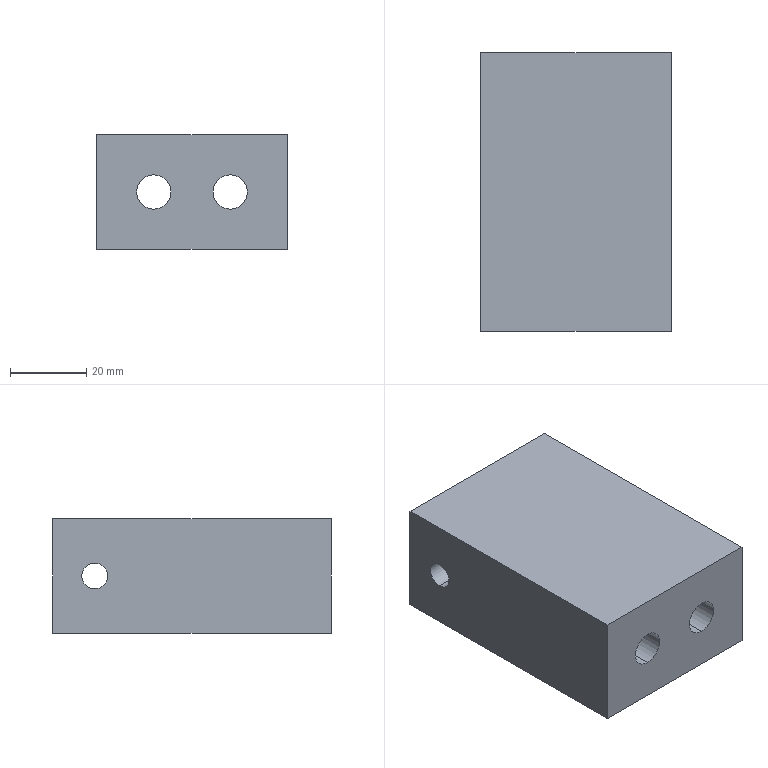Part | STEP file | HXGR200008-05-02 | 1 solid | 22 faces | box 50 x 73 x 30 mm | volume 90409 mm3 | cylinder 14 | plane 8 | commonest cylinder face diameters 6.8 x6 9 x4 15 x4
STEP:
#1=CARTESIAN_POINT('',(25.,25.5,-3.4));
#2=VERTEX_POINT('',#1);
#3=CARTESIAN_POINT('',(25.,25.5,3.4));
#4=VERTEX_POINT('',#3);
#5=CARTESIAN_POINT('',(25.,25.5,0.));
#6=DIRECTION('',(-1.,0.,0.));
#7=DIRECTION('',(0.,0.,1.));
#8=AXIS2_PLACEMENT_3D('',#5,#6,#7);
#9=CIRCLE('',#8,3.4);
#10=EDGE_CURVE('',#2,#4,#9,.T.);
#11=ORIENTED_EDGE('',*,*,#10,.F.);
#12=CARTESIAN_POINT('',(16.685,25.5,-3.4));
#13=VERTEX_POINT('',#12);
#14=CARTESIAN_POINT('',(-25.,25.5,-3.4));
#15=DIRECTION('',(-1.,0.,0.));
#16=VECTOR('',#15,1000.);
#17=LINE('',#14,#16);
#18=EDGE_CURVE('',#2,#13,#17,.T.);
#19=ORIENTED_EDGE('',*,*,#18,.T.);
#20=CARTESIAN_POINT('',(16.685,25.5,3.4));
#21=VERTEX_POINT('',#20);
#22=CARTESIAN_POINT('',(16.685,25.5,3.4));
#23=CARTESIAN_POINT('',(16.685,25.272,3.4));
#24=CARTESIAN_POINT('',(16.697,25.048,3.377));
#25=CARTESIAN_POINT('',(16.741,24.61,3.289));
#26=CARTESIAN_POINT('',(16.773,24.392,3.222));
#27=CARTESIAN_POINT('',(16.852,23.983,3.051));
#28=CARTESIAN_POINT('',(16.898,23.789,2.946));
#29=CARTESIAN_POINT('',(16.998,23.422,2.7));
#30=CARTESIAN_POINT('',(17.052,23.251,2.559));
#31=CARTESIAN_POINT('',(17.156,22.942,2.25));
#32=CARTESIAN_POINT('',(17.209,22.801,2.079));
#33=CARTESIAN_POINT('',(17.305,22.554,1.711));
#34=CARTESIAN_POINT('',(17.348,22.449,1.517));
#35=CARTESIAN_POINT('',(17.421,22.278,1.109));
#36=CARTESIAN_POINT('',(17.45,22.211,0.8911));
#37=CARTESIAN_POINT('',(17.49,22.122,0.4505));
#38=CARTESIAN_POINT('',(17.5,22.1,0.2275));
#39=CARTESIAN_POINT('',(17.5,22.1,-0.2236));
#40=CARTESIAN_POINT('',(17.49,22.123,-0.452));
#41=CARTESIAN_POINT('',(17.45,22.211,-0.8913));
#42=CARTESIAN_POINT('',(17.421,22.277,-1.106));
#43=CARTESIAN_POINT('',(17.347,22.45,-1.52));
#44=CARTESIAN_POINT('',(17.304,22.556,-1.715));
#45=CARTESIAN_POINT('',(17.208,22.802,-2.08));
#46=CARTESIAN_POINT('',(17.156,22.944,-2.253));
#47=CARTESIAN_POINT('',(17.051,23.254,-2.562));
#48=CARTESIAN_POINT('',(16.998,23.423,-2.701));
#49=CARTESIAN_POINT('',(16.898,23.79,-2.947));
#50=CARTESIAN_POINT('',(16.851,23.987,-3.053));
#51=CARTESIAN_POINT('',(16.773,24.394,-3.223));
#52=CARTESIAN_POINT('',(16.741,24.607,-3.289));
#53=CARTESIAN_POINT('',(16.696,25.052,-3.378));
#54=CARTESIAN_POINT('',(16.685,25.275,-3.4));
#55=CARTESIAN_POINT('',(16.685,25.5,-3.4));
#56=B_SPLINE_CURVE_WITH_KNOTS('',3,(#22,#23,#24,#25,#26,#27,#28,#29,#30,#31,#32,#33,#34,#35,#36,#37,#38,#39,#40,#41,#42,#43,#44,#45,#46,#47,#48,#49,#50,#51,#52,#53,#54,#55),.UNSPECIFIED.,.F.,.F.,(4,2,2,2,2,2,2,2,2,2,2,2,2,2,2,2,4),(0.,0.0006736,0.001347,0.002021,0.002695,0.003368,0.004042,0.004715,0.005389,0.006063,0.006736,0.00741,0.008084,0.008757,0.009431,0.0101,0.01078),.UNSPECIFIED.);
#57=EDGE_CURVE('',#21,#13,#56,.T.);
#58=ORIENTED_EDGE('',*,*,#57,.F.);
#59=CARTESIAN_POINT('',(-25.,25.5,3.4));
#60=DIRECTION('',(-1.,0.,0.));
#61=VECTOR('',#60,1000.);
#62=LINE('',#59,#61);
#63=EDGE_CURVE('',#4,#21,#62,.T.);
#64=ORIENTED_EDGE('',*,*,#63,.F.);
#65=EDGE_LOOP('',(#11,#19,#58,#64));
#66=FACE_OUTER_BOUND('',#65,.T.);
#67=CARTESIAN_POINT('',(-25.,25.5,0.));
#68=DIRECTION('',(-1.,0.,0.));
#69=DIRECTION('',(0.,0.,1.));
#70=AXIS2_PLACEMENT_3D('',#67,#68,#69);
#71=CYLINDRICAL_SURFACE('',#70,3.4);
#72=ADVANCED_FACE('',(#66),#71,.F.);
#73=CARTESIAN_POINT('',(-16.685,25.5,-3.4));
#74=VERTEX_POINT('',#73);
#75=CARTESIAN_POINT('',(-16.685,25.5,3.4));
#76=VERTEX_POINT('',#75);
#77=CARTESIAN_POINT('',(-16.685,25.5,-3.4));
#78=CARTESIAN_POINT('',(-16.685,25.276,-3.4));
#79=CARTESIAN_POINT('',(-16.697,25.048,-3.377));
#80=CARTESIAN_POINT('',(-16.741,24.607,-3.288));
#81=CARTESIAN_POINT('',(-16.773,24.394,-3.223));
#82=CARTESIAN_POINT('',(-16.852,23.983,-3.051));
#83=CARTESIAN_POINT('',(-16.899,23.787,-2.945));
#84=CARTESIAN_POINT('',(-16.998,23.422,-2.7));
#85=CARTESIAN_POINT('',(-17.052,23.251,-2.559));
#86=CARTESIAN_POINT('',(-17.157,22.94,-2.248));
#87=CARTESIAN_POINT('',(-17.208,22.801,-2.079));
#88=CARTESIAN_POINT('',(-17.304,22.556,-1.714));
#89=CARTESIAN_POINT('',(-17.348,22.449,-1.516));
#90=CARTESIAN_POINT('',(-17.421,22.278,-1.107));
#91=CARTESIAN_POINT('',(-17.45,22.212,-0.8946));
#92=CARTESIAN_POINT('',(-17.49,22.123,-0.4535));
#93=CARTESIAN_POINT('',(-17.5,22.1,-0.2259));
#94=CARTESIAN_POINT('',(-17.5,22.1,0.223));
#95=CARTESIAN_POINT('',(-17.49,22.122,0.4485));
#96=CARTESIAN_POINT('',(-17.45,22.211,0.8921));
#97=CARTESIAN_POINT('',(-17.421,22.277,1.105));
#98=CARTESIAN_POINT('',(-17.348,22.449,1.516));
#99=CARTESIAN_POINT('',(-17.304,22.556,1.714));
#100=CARTESIAN_POINT('',(-17.208,22.801,2.08));
#101=CARTESIAN_POINT('',(-17.157,22.94,2.249));
#102=CARTESIAN_POINT('',(-17.051,23.253,2.561));
#103=CARTESIAN_POINT('',(-16.998,23.423,2.701));
#104=CARTESIAN_POINT('',(-16.899,23.787,2.945));
#105=CARTESIAN_POINT('',(-16.852,23.983,3.051));
#106=CARTESIAN_POINT('',(-16.773,24.394,3.223));
#107=CARTESIAN_POINT('',(-16.741,24.606,3.288));
#108=CARTESIAN_POINT('',(-16.697,25.044,3.377));
#109=CARTESIAN_POINT('',(-16.685,25.272,3.4));
#110=CARTESIAN_POINT('',(-16.685,25.5,3.4));
#111=B_SPLINE_CURVE_WITH_KNOTS('',3,(#77,#78,#79,#80,#81,#82,#83,#84,#85,#86,#87,#88,#89,#90,#91,#92,#93,#94,#95,#96,#97,#98,#99,#100,#101,#102,#103,#104,#105,#106,#107,#108,#109,#110),.UNSPECIFIED.,.F.,.F.,(4,2,2,2,2,2,2,2,2,2,2,2,2,2,2,2,4),(0.01078,0.01145,0.01212,0.0128,0.01347,0.01414,0.01482,0.01549,0.01616,0.01683,0.01751,0.01818,0.01885,0.01953,0.0202,0.02087,0.02154),.UNSPECIFIED.);
#112=EDGE_CURVE('',#74,#76,#111,.T.);
#113=ORIENTED_EDGE('',*,*,#112,.F.);
#114=CARTESIAN_POINT('',(-25.,25.5,-3.4));
#115=VERTEX_POINT('',#114);
#116=CARTESIAN_POINT('',(-25.,25.5,-3.4));
#117=DIRECTION('',(-1.,0.,0.));
#118=VECTOR('',#117,1000.);
#119=LINE('',#116,#118);
#120=EDGE_CURVE('',#74,#115,#119,.T.);
#121=ORIENTED_EDGE('',*,*,#120,.T.);
#122=CARTESIAN_POINT('',(-25.,25.5,3.4));
#123=VERTEX_POINT('',#122);
#124=CARTESIAN_POINT('',(-25.,25.5,0.));
#125=DIRECTION('',(-1.,0.,0.));
#126=DIRECTION('',(0.,0.,1.));
#127=AXIS2_PLACEMENT_3D('',#124,#125,#126);
#128=CIRCLE('',#127,3.4);
#129=EDGE_CURVE('',#115,#123,#128,.T.);
#130=ORIENTED_EDGE('',*,*,#129,.T.);
#131=CARTESIAN_POINT('',(-25.,25.5,3.4));
#132=DIRECTION('',(-1.,0.,0.));
#133=VECTOR('',#132,1000.);
#134=LINE('',#131,#133);
#135=EDGE_CURVE('',#76,#123,#134,.T.);
#136=ORIENTED_EDGE('',*,*,#135,.F.);
#137=EDGE_LOOP('',(#113,#121,#130,#136));
#138=FACE_OUTER_BOUND('',#137,.T.);
#139=CARTESIAN_POINT('',(-25.,25.5,0.));
#140=DIRECTION('',(-1.,0.,0.));
#141=DIRECTION('',(0.,0.,1.));
#142=AXIS2_PLACEMENT_3D('',#139,#140,#141);
#143=CYLINDRICAL_SURFACE('',#142,3.4);
#144=ADVANCED_FACE('',(#138),#143,.F.);
#145=CARTESIAN_POINT('',(3.315,25.5,-3.4));
#146=VERTEX_POINT('',#145);
#147=CARTESIAN_POINT('',(3.315,25.5,3.4));
#148=VERTEX_POINT('',#147);
#149=CARTESIAN_POINT('',(3.315,25.5,-3.4));
#150=CARTESIAN_POINT('',(3.315,25.276,-3.4));
#151=CARTESIAN_POINT('',(3.303,25.048,-3.377));
#152=CARTESIAN_POINT('',(3.259,24.607,-3.288));
#153=CARTESIAN_POINT('',(3.227,24.394,-3.223));
#154=CARTESIAN_POINT('',(3.148,23.983,-3.051));
#155=CARTESIAN_POINT('',(3.101,23.787,-2.945));
#156=CARTESIAN_POINT('',(3.002,23.422,-2.7));
#157=CARTESIAN_POINT('',(2.948,23.251,-2.559));
#158=CARTESIAN_POINT('',(2.843,22.94,-2.248));
#159=CARTESIAN_POINT('',(2.792,22.801,-2.079));
#160=CARTESIAN_POINT('',(2.696,22.556,-1.714));
#161=CARTESIAN_POINT('',(2.652,22.449,-1.516));
#162=CARTESIAN_POINT('',(2.579,22.278,-1.107));
#163=CARTESIAN_POINT('',(2.55,22.212,-0.8946));
#164=CARTESIAN_POINT('',(2.51,22.123,-0.4535));
#165=CARTESIAN_POINT('',(2.5,22.1,-0.2259));
#166=CARTESIAN_POINT('',(2.5,22.1,0.223));
#167=CARTESIAN_POINT('',(2.51,22.122,0.4485));
#168=CARTESIAN_POINT('',(2.55,22.211,0.8921));
#169=CARTESIAN_POINT('',(2.579,22.277,1.105));
#170=CARTESIAN_POINT('',(2.652,22.449,1.516));
#171=CARTESIAN_POINT('',(2.696,22.556,1.714));
#172=CARTESIAN_POINT('',(2.792,22.801,2.08));
#173=CARTESIAN_POINT('',(2.843,22.94,2.249));
#174=CARTESIAN_POINT('',(2.949,23.253,2.561));
#175=CARTESIAN_POINT('',(3.002,23.423,2.701));
#176=CARTESIAN_POINT('',(3.101,23.787,2.945));
#177=CARTESIAN_POINT('',(3.148,23.983,3.051));
#178=CARTESIAN_POINT('',(3.227,24.394,3.223));
#179=CARTESIAN_POINT('',(3.259,24.606,3.288));
#180=CARTESIAN_POINT('',(3.303,25.044,3.377));
#181=CARTESIAN_POINT('',(3.315,25.272,3.4));
#182=CARTESIAN_POINT('',(3.315,25.5,3.4));
#183=B_SPLINE_CURVE_WITH_KNOTS('',3,(#149,#150,#151,#152,#153,#154,#155,#156,#157,#158,#159,#160,#161,#162,#163,#164,#165,#166,#167,#168,#169,#170,#171,#172,#173,#174,#175,#176,#177,#178,#179,#180,#181,#182),.UNSPECIFIED.,.F.,.F.,(4,2,2,2,2,2,2,2,2,2,2,2,2,2,2,2,4),(0.01078,0.01145,0.01212,0.0128,0.01347,0.01414,0.01482,0.01549,0.01616,0.01683,0.01751,0.01818,0.01885,0.01953,0.0202,0.02087,0.02154),.UNSPECIFIED.);
#184=EDGE_CURVE('',#146,#148,#183,.T.);
#185=ORIENTED_EDGE('',*,*,#184,.F.);
#186=CARTESIAN_POINT('',(-3.315,25.5,-3.4));
#187=VERTEX_POINT('',#186);
#188=CARTESIAN_POINT('',(-25.,25.5,-3.4));
#189=DIRECTION('',(-1.,0.,0.));
#190=VECTOR('',#189,1000.);
#191=LINE('',#188,#190);
#192=EDGE_CURVE('',#146,#187,#191,.T.);
#193=ORIENTED_EDGE('',*,*,#192,.T.);
#194=CARTESIAN_POINT('',(-3.315,25.5,3.4));
#195=VERTEX_POINT('',#194);
#196=CARTESIAN_POINT('',(-3.315,25.5,3.4));
#197=CARTESIAN_POINT('',(-3.315,25.272,3.4));
#198=CARTESIAN_POINT('',(-3.303,25.048,3.377));
#199=CARTESIAN_POINT('',(-3.259,24.61,3.289));
#200=CARTESIAN_POINT('',(-3.227,24.392,3.222));
#201=CARTESIAN_POINT('',(-3.148,23.983,3.051));
#202=CARTESIAN_POINT('',(-3.102,23.789,2.946));
#203=CARTESIAN_POINT('',(-3.002,23.422,2.7));
#204=CARTESIAN_POINT('',(-2.948,23.251,2.559));
#205=CARTESIAN_POINT('',(-2.844,22.942,2.25));
#206=CARTESIAN_POINT('',(-2.791,22.801,2.079));
#207=CARTESIAN_POINT('',(-2.695,22.554,1.711));
#208=CARTESIAN_POINT('',(-2.652,22.449,1.517));
#209=CARTESIAN_POINT('',(-2.579,22.278,1.109));
#210=CARTESIAN_POINT('',(-2.55,22.211,0.8911));
#211=CARTESIAN_POINT('',(-2.51,22.122,0.4505));
#212=CARTESIAN_POINT('',(-2.5,22.1,0.2275));
#213=CARTESIAN_POINT('',(-2.5,22.1,-0.2236));
#214=CARTESIAN_POINT('',(-2.51,22.123,-0.452));
#215=CARTESIAN_POINT('',(-2.55,22.211,-0.8913));
#216=CARTESIAN_POINT('',(-2.579,22.277,-1.106));
#217=CARTESIAN_POINT('',(-2.653,22.45,-1.52));
#218=CARTESIAN_POINT('',(-2.696,22.556,-1.715));
#219=CARTESIAN_POINT('',(-2.792,22.802,-2.08));
#220=CARTESIAN_POINT('',(-2.844,22.944,-2.253));
#221=CARTESIAN_POINT('',(-2.949,23.254,-2.562));
#222=CARTESIAN_POINT('',(-3.002,23.423,-2.701));
#223=CARTESIAN_POINT('',(-3.102,23.79,-2.947));
#224=CARTESIAN_POINT('',(-3.149,23.987,-3.053));
#225=CARTESIAN_POINT('',(-3.227,24.394,-3.223));
#226=CARTESIAN_POINT('',(-3.259,24.607,-3.289));
#227=CARTESIAN_POINT('',(-3.304,25.052,-3.378));
#228=CARTESIAN_POINT('',(-3.315,25.275,-3.4));
#229=CARTESIAN_POINT('',(-3.315,25.5,-3.4));
#230=B_SPLINE_CURVE_WITH_KNOTS('',3,(#196,#197,#198,#199,#200,#201,#202,#203,#204,#205,#206,#207,#208,#209,#210,#211,#212,#213,#214,#215,#216,#217,#218,#219,#220,#221,#222,#223,#224,#225,#226,#227,#228,#229),.UNSPECIFIED.,.F.,.F.,(4,2,2,2,2,2,2,2,2,2,2,2,2,2,2,2,4),(0.,0.0006736,0.001347,0.002021,0.002695,0.003368,0.004042,0.004715,0.005389,0.006063,0.006736,0.00741,0.008084,0.008757,0.009431,0.0101,0.01078),.UNSPECIFIED.);
#231=EDGE_CURVE('',#195,#187,#230,.T.);
#232=ORIENTED_EDGE('',*,*,#231,.F.);
#233=CARTESIAN_POINT('',(-25.,25.5,3.4));
#234=DIRECTION('',(-1.,0.,0.));
#235=VECTOR('',#234,1000.);
#236=LINE('',#233,#235);
#237=EDGE_CURVE('',#148,#195,#236,.T.);
#238=ORIENTED_EDGE('',*,*,#237,.F.);
#239=EDGE_LOOP('',(#185,#193,#232,#238));
#240=FACE_OUTER_BOUND('',#239,.T.);
#241=CARTESIAN_POINT('',(-25.,25.5,0.));
#242=DIRECTION('',(-1.,0.,0.));
#243=DIRECTION('',(0.,0.,1.));
#244=AXIS2_PLACEMENT_3D('',#241,#242,#243);
#245=CYLINDRICAL_SURFACE('',#244,3.4);
#246=ADVANCED_FACE('',(#240),#245,.F.);
#247=CARTESIAN_POINT('',(-16.685,25.5,3.4));
#248=CARTESIAN_POINT('',(-16.685,25.728,3.4));
#249=CARTESIAN_POINT('',(-16.697,25.952,3.377));
#250=CARTESIAN_POINT('',(-16.741,26.39,3.289));
#251=CARTESIAN_POINT('',(-16.773,26.608,3.222));
#252=CARTESIAN_POINT('',(-16.852,27.017,3.051));
#253=CARTESIAN_POINT('',(-16.898,27.211,2.946));
#254=CARTESIAN_POINT('',(-16.998,27.578,2.7));
#255=CARTESIAN_POINT('',(-17.052,27.749,2.559));
#256=CARTESIAN_POINT('',(-17.156,28.058,2.25));
#257=CARTESIAN_POINT('',(-17.209,28.199,2.079));
#258=CARTESIAN_POINT('',(-17.305,28.446,1.711));
#259=CARTESIAN_POINT('',(-17.348,28.551,1.517));
#260=CARTESIAN_POINT('',(-17.421,28.722,1.109));
#261=CARTESIAN_POINT('',(-17.45,28.789,0.8911));
#262=CARTESIAN_POINT('',(-17.49,28.878,0.4505));
#263=CARTESIAN_POINT('',(-17.5,28.9,0.2275));
#264=CARTESIAN_POINT('',(-17.5,28.9,-0.2236));
#265=CARTESIAN_POINT('',(-17.49,28.877,-0.452));
#266=CARTESIAN_POINT('',(-17.45,28.789,-0.8913));
#267=CARTESIAN_POINT('',(-17.421,28.723,-1.106));
#268=CARTESIAN_POINT('',(-17.347,28.55,-1.52));
#269=CARTESIAN_POINT('',(-17.304,28.444,-1.715));
#270=CARTESIAN_POINT('',(-17.208,28.198,-2.08));
#271=CARTESIAN_POINT('',(-17.156,28.056,-2.253));
#272=CARTESIAN_POINT('',(-17.051,27.746,-2.562));
#273=CARTESIAN_POINT('',(-16.998,27.577,-2.701));
#274=CARTESIAN_POINT('',(-16.898,27.21,-2.947));
#275=CARTESIAN_POINT('',(-16.851,27.013,-3.053));
#276=CARTESIAN_POINT('',(-16.773,26.606,-3.223));
#277=CARTESIAN_POINT('',(-16.741,26.393,-3.289));
#278=CARTESIAN_POINT('',(-16.696,25.948,-3.378));
#279=CARTESIAN_POINT('',(-16.685,25.725,-3.4));
#280=CARTESIAN_POINT('',(-16.685,25.5,-3.4));
#281=B_SPLINE_CURVE_WITH_KNOTS('',3,(#247,#248,#249,#250,#251,#252,#253,#254,#255,#256,#257,#258,#259,#260,#261,#262,#263,#264,#265,#266,#267,#268,#269,#270,#271,#272,#273,#274,#275,#276,#277,#278,#279,#280),.UNSPECIFIED.,.F.,.F.,(4,2,2,2,2,2,2,2,2,2,2,2,2,2,2,2,4),(0.,0.0006736,0.001347,0.002021,0.002695,0.003368,0.004042,0.004715,0.005389,0.006063,0.006736,0.00741,0.008084,0.008757,0.009431,0.0101,0.01078),.UNSPECIFIED.);
#282=EDGE_CURVE('',#76,#74,#281,.T.);
#283=ORIENTED_EDGE('',*,*,#282,.T.);
#284=ORIENTED_EDGE('',*,*,#112,.T.);
#285=EDGE_LOOP('',(#283,#284));
#286=FACE_BOUND('',#285,.T.);
#287=CARTESIAN_POINT('',(-10.,-3.5,-7.5));
#288=VERTEX_POINT('',#287);
#289=CARTESIAN_POINT('',(-10.,-3.5,7.5));
#290=VERTEX_POINT('',#289);
#291=CARTESIAN_POINT('',(-10.,-3.5,0.));
#292=DIRECTION('',(0.,1.,0.));
#293=DIRECTION('',(0.,0.,1.));
#294=AXIS2_PLACEMENT_3D('',#291,#292,#293);
#295=CIRCLE('',#294,7.5);
#296=EDGE_CURVE('',#288,#290,#295,.T.);
#297=ORIENTED_EDGE('',*,*,#296,.F.);
#298=CARTESIAN_POINT('',(-10.,36.5,-7.5));
#299=VERTEX_POINT('',#298);
#300=CARTESIAN_POINT('',(-10.,36.5,-7.5));
#301=DIRECTION('',(0.,1.,0.));
#302=VECTOR('',#301,1000.);
#303=LINE('',#300,#302);
#304=EDGE_CURVE('',#288,#299,#303,.T.);
#305=ORIENTED_EDGE('',*,*,#304,.T.);
#306=CARTESIAN_POINT('',(-10.,36.5,7.5));
#307=VERTEX_POINT('',#306);
#308=CARTESIAN_POINT('',(-10.,36.5,0.));
#309=DIRECTION('',(0.,1.,0.));
#310=DIRECTION('',(0.,0.,1.));
#311=AXIS2_PLACEMENT_3D('',#308,#309,#310);
#312=CIRCLE('',#311,7.5);
#313=EDGE_CURVE('',#299,#307,#312,.T.);
#314=ORIENTED_EDGE('',*,*,#313,.T.);
#315=CARTESIAN_POINT('',(-10.,36.5,7.5));
#316=DIRECTION('',(0.,1.,0.));
#317=VECTOR('',#316,1000.);
#318=LINE('',#315,#317);
#319=EDGE_CURVE('',#290,#307,#318,.T.);
#320=ORIENTED_EDGE('',*,*,#319,.F.);
#321=EDGE_LOOP('',(#297,#305,#314,#320));
#322=FACE_OUTER_BOUND('',#321,.T.);
#323=CARTESIAN_POINT('',(-10.,36.5,0.));
#324=DIRECTION('',(0.,1.,0.));
#325=DIRECTION('',(0.,0.,1.));
#326=AXIS2_PLACEMENT_3D('',#323,#324,#325);
#327=CYLINDRICAL_SURFACE('',#326,7.5);
#328=ADVANCED_FACE('',(#286,#322),#327,.F.);
#329=CARTESIAN_POINT('',(-10.,-36.5,-4.5));
#330=VERTEX_POINT('',#329);
#331=CARTESIAN_POINT('',(-10.,-36.5,4.5));
#332=VERTEX_POINT('',#331);
#333=CARTESIAN_POINT('',(-10.,-36.5,0.));
#334=DIRECTION('',(0.,1.,0.));
#335=DIRECTION('',(0.,0.,1.));
#336=AXIS2_PLACEMENT_3D('',#333,#334,#335);
#337=CIRCLE('',#336,4.5);
#338=EDGE_CURVE('',#330,#332,#337,.T.);
#339=ORIENTED_EDGE('',*,*,#338,.F.);
#340=CARTESIAN_POINT('',(-10.,-3.5,-4.5));
#341=VERTEX_POINT('',#340);
#342=CARTESIAN_POINT('',(-10.,36.5,-4.5));
#343=DIRECTION('',(0.,1.,0.));
#344=VECTOR('',#343,1000.);
#345=LINE('',#342,#344);
#346=EDGE_CURVE('',#330,#341,#345,.T.);
#347=ORIENTED_EDGE('',*,*,#346,.T.);
#348=CARTESIAN_POINT('',(-10.,-3.5,4.5));
#349=VERTEX_POINT('',#348);
#350=CARTESIAN_POINT('',(-10.,-3.5,0.));
#351=DIRECTION('',(0.,1.,0.));
#352=DIRECTION('',(0.,0.,1.));
#353=AXIS2_PLACEMENT_3D('',#350,#351,#352);
#354=CIRCLE('',#353,4.5);
#355=EDGE_CURVE('',#341,#349,#354,.T.);
#356=ORIENTED_EDGE('',*,*,#355,.T.);
#357=CARTESIAN_POINT('',(-10.,36.5,4.5));
#358=DIRECTION('',(0.,1.,0.));
#359=VECTOR('',#358,1000.);
#360=LINE('',#357,#359);
#361=EDGE_CURVE('',#332,#349,#360,.T.);
#362=ORIENTED_EDGE('',*,*,#361,.F.);
#363=EDGE_LOOP('',(#339,#347,#356,#362));
#364=FACE_OUTER_BOUND('',#363,.T.);
#365=CARTESIAN_POINT('',(-10.,36.5,0.));
#366=DIRECTION('',(0.,1.,0.));
#367=DIRECTION('',(0.,0.,1.));
#368=AXIS2_PLACEMENT_3D('',#365,#366,#367);
#369=CYLINDRICAL_SURFACE('',#368,4.5);
#370=ADVANCED_FACE('',(#364),#369,.F.);
#371=CARTESIAN_POINT('',(3.315,25.5,3.4));
#372=CARTESIAN_POINT('',(3.315,25.728,3.4));
#373=CARTESIAN_POINT('',(3.303,25.952,3.377));
#374=CARTESIAN_POINT('',(3.259,26.39,3.289));
#375=CARTESIAN_POINT('',(3.227,26.608,3.222));
#376=CARTESIAN_POINT('',(3.148,27.017,3.051));
#377=CARTESIAN_POINT('',(3.102,27.211,2.946));
#378=CARTESIAN_POINT('',(3.002,27.578,2.7));
#379=CARTESIAN_POINT('',(2.948,27.749,2.559));
#380=CARTESIAN_POINT('',(2.844,28.058,2.25));
#381=CARTESIAN_POINT('',(2.791,28.199,2.079));
#382=CARTESIAN_POINT('',(2.695,28.446,1.711));
#383=CARTESIAN_POINT('',(2.652,28.551,1.517));
#384=CARTESIAN_POINT('',(2.579,28.722,1.109));
#385=CARTESIAN_POINT('',(2.55,28.789,0.8911));
#386=CARTESIAN_POINT('',(2.51,28.878,0.4505));
#387=CARTESIAN_POINT('',(2.5,28.9,0.2275));
#388=CARTESIAN_POINT('',(2.5,28.9,-0.2236));
#389=CARTESIAN_POINT('',(2.51,28.877,-0.452));
#390=CARTESIAN_POINT('',(2.55,28.789,-0.8913));
#391=CARTESIAN_POINT('',(2.579,28.723,-1.106));
#392=CARTESIAN_POINT('',(2.653,28.55,-1.52));
#393=CARTESIAN_POINT('',(2.696,28.444,-1.715));
#394=CARTESIAN_POINT('',(2.792,28.198,-2.08));
#395=CARTESIAN_POINT('',(2.844,28.056,-2.253));
#396=CARTESIAN_POINT('',(2.949,27.746,-2.562));
#397=CARTESIAN_POINT('',(3.002,27.577,-2.701));
#398=CARTESIAN_POINT('',(3.102,27.21,-2.947));
#399=CARTESIAN_POINT('',(3.149,27.013,-3.053));
#400=CARTESIAN_POINT('',(3.227,26.606,-3.223));
#401=CARTESIAN_POINT('',(3.259,26.393,-3.289));
#402=CARTESIAN_POINT('',(3.304,25.948,-3.378));
#403=CARTESIAN_POINT('',(3.315,25.725,-3.4));
#404=CARTESIAN_POINT('',(3.315,25.5,-3.4));
#405=B_SPLINE_CURVE_WITH_KNOTS('',3,(#371,#372,#373,#374,#375,#376,#377,#378,#379,#380,#381,#382,#383,#384,#385,#386,#387,#388,#389,#390,#391,#392,#393,#394,#395,#396,#397,#398,#399,#400,#401,#402,#403,#404),.UNSPECIFIED.,.F.,.F.,(4,2,2,2,2,2,2,2,2,2,2,2,2,2,2,2,4),(0.,0.0006736,0.001347,0.002021,0.002695,0.003368,0.004042,0.004715,0.005389,0.006063,0.006736,0.00741,0.008084,0.008757,0.009431,0.0101,0.01078),.UNSPECIFIED.);
#406=EDGE_CURVE('',#148,#146,#405,.T.);
#407=ORIENTED_EDGE('',*,*,#406,.T.);
#408=ORIENTED_EDGE('',*,*,#184,.T.);
#409=EDGE_LOOP('',(#407,#408));
#410=FACE_BOUND('',#409,.T.);
#411=CARTESIAN_POINT('',(10.,-3.5,-7.5));
#412=VERTEX_POINT('',#411);
#413=CARTESIAN_POINT('',(10.,-3.5,7.5));
#414=VERTEX_POINT('',#413);
#415=CARTESIAN_POINT('',(10.,-3.5,0.));
#416=DIRECTION('',(0.,1.,0.));
#417=DIRECTION('',(0.,0.,1.));
#418=AXIS2_PLACEMENT_3D('',#415,#416,#417);
#419=CIRCLE('',#418,7.5);
#420=EDGE_CURVE('',#412,#414,#419,.T.);
#421=ORIENTED_EDGE('',*,*,#420,.F.);
#422=CARTESIAN_POINT('',(10.,36.5,-7.5));
#423=VERTEX_POINT('',#422);
#424=CARTESIAN_POINT('',(10.,36.5,-7.5));
#425=DIRECTION('',(0.,1.,0.));
#426=VECTOR('',#425,1000.);
#427=LINE('',#424,#426);
#428=EDGE_CURVE('',#412,#423,#427,.T.);
#429=ORIENTED_EDGE('',*,*,#428,.T.);
#430=CARTESIAN_POINT('',(10.,36.5,7.5));
#431=VERTEX_POINT('',#430);
#432=CARTESIAN_POINT('',(10.,36.5,0.));
#433=DIRECTION('',(0.,1.,0.));
#434=DIRECTION('',(0.,0.,1.));
#435=AXIS2_PLACEMENT_3D('',#432,#433,#434);
#436=CIRCLE('',#435,7.5);
#437=EDGE_CURVE('',#423,#431,#436,.T.);
#438=ORIENTED_EDGE('',*,*,#437,.T.);
#439=CARTESIAN_POINT('',(10.,36.5,7.5));
#440=DIRECTION('',(0.,1.,0.));
#441=VECTOR('',#440,1000.);
#442=LINE('',#439,#441);
#443=EDGE_CURVE('',#414,#431,#442,.T.);
#444=ORIENTED_EDGE('',*,*,#443,.F.);
#445=EDGE_LOOP('',(#421,#429,#438,#444));
#446=FACE_OUTER_BOUND('',#445,.T.);
#447=CARTESIAN_POINT('',(10.,36.5,0.));
#448=DIRECTION('',(0.,1.,0.));
#449=DIRECTION('',(0.,0.,1.));
#450=AXIS2_PLACEMENT_3D('',#447,#448,#449);
#451=CYLINDRICAL_SURFACE('',#450,7.5);
#452=ADVANCED_FACE('',(#410,#446),#451,.F.);
#453=CARTESIAN_POINT('',(10.,-36.5,-4.5));
#454=VERTEX_POINT('',#453);
#455=CARTESIAN_POINT('',(10.,-36.5,4.5));
#456=VERTEX_POINT('',#455);
#457=CARTESIAN_POINT('',(10.,-36.5,0.));
#458=DIRECTION('',(0.,1.,0.));
#459=DIRECTION('',(0.,0.,1.));
#460=AXIS2_PLACEMENT_3D('',#457,#458,#459);
#461=CIRCLE('',#460,4.5);
#462=EDGE_CURVE('',#454,#456,#461,.T.);
#463=ORIENTED_EDGE('',*,*,#462,.F.);
#464=CARTESIAN_POINT('',(10.,-3.5,-4.5));
#465=VERTEX_POINT('',#464);
#466=CARTESIAN_POINT('',(10.,36.5,-4.5));
#467=DIRECTION('',(0.,1.,0.));
#468=VECTOR('',#467,1000.);
#469=LINE('',#466,#468);
#470=EDGE_CURVE('',#454,#465,#469,.T.);
#471=ORIENTED_EDGE('',*,*,#470,.T.);
#472=CARTESIAN_POINT('',(10.,-3.5,4.5));
#473=VERTEX_POINT('',#472);
#474=CARTESIAN_POINT('',(10.,-3.5,0.));
#475=DIRECTION('',(0.,1.,0.));
#476=DIRECTION('',(0.,0.,1.));
#477=AXIS2_PLACEMENT_3D('',#474,#475,#476);
#478=CIRCLE('',#477,4.5);
#479=EDGE_CURVE('',#465,#473,#478,.T.);
#480=ORIENTED_EDGE('',*,*,#479,.T.);
#481=CARTESIAN_POINT('',(10.,36.5,4.5));
#482=DIRECTION('',(0.,1.,0.));
#483=VECTOR('',#482,1000.);
#484=LINE('',#481,#483);
#485=EDGE_CURVE('',#456,#473,#484,.T.);
#486=ORIENTED_EDGE('',*,*,#485,.F.);
#487=EDGE_LOOP('',(#463,#471,#480,#486));
#488=FACE_OUTER_BOUND('',#487,.T.);
#489=CARTESIAN_POINT('',(10.,36.5,0.));
#490=DIRECTION('',(0.,1.,0.));
#491=DIRECTION('',(0.,0.,1.));
#492=AXIS2_PLACEMENT_3D('',#489,#490,#491);
#493=CYLINDRICAL_SURFACE('',#492,4.5);
#494=ADVANCED_FACE('',(#488),#493,.F.);
#495=CARTESIAN_POINT('',(-25.,25.5,0.));
#496=DIRECTION('',(-1.,0.,0.));
#497=DIRECTION('',(0.,0.,1.));
#498=AXIS2_PLACEMENT_3D('',#495,#496,#497);
#499=CIRCLE('',#498,3.4);
#500=EDGE_CURVE('',#123,#115,#499,.T.);
#501=ORIENTED_EDGE('',*,*,#500,.F.);
#502=ORIENTED_EDGE('',*,*,#129,.F.);
#503=EDGE_LOOP('',(#501,#502));
#504=FACE_BOUND('',#503,.T.);
#505=CARTESIAN_POINT('',(-25.,36.5,-15.));
#506=VERTEX_POINT('',#505);
#507=CARTESIAN_POINT('',(-25.,-36.5,-15.));
#508=VERTEX_POINT('',#507);
#509=CARTESIAN_POINT('',(-25.,-36.5,-15.));
#510=DIRECTION('',(0.,-1.,0.));
#511=VECTOR('',#510,1000.);
#512=LINE('',#509,#511);
#513=EDGE_CURVE('',#506,#508,#512,.T.);
#514=ORIENTED_EDGE('',*,*,#513,.T.);
#515=CARTESIAN_POINT('',(-25.,-36.5,15.));
#516=VERTEX_POINT('',#515);
#517=CARTESIAN_POINT('',(-25.,-36.5,15.));
#518=DIRECTION('',(0.,0.,-1.));
#519=VECTOR('',#518,1000.);
#520=LINE('',#517,#519);
#521=EDGE_CURVE('',#516,#508,#520,.T.);
#522=ORIENTED_EDGE('',*,*,#521,.F.);
#523=CARTESIAN_POINT('',(-25.,36.5,15.));
#524=VERTEX_POINT('',#523);
#525=CARTESIAN_POINT('',(-25.,-36.5,15.));
#526=DIRECTION('',(0.,-1.,0.));
#527=VECTOR('',#526,1000.);
#528=LINE('',#525,#527);
#529=EDGE_CURVE('',#524,#516,#528,.T.);
#530=ORIENTED_EDGE('',*,*,#529,.F.);
#531=CARTESIAN_POINT('',(-25.,36.5,15.));
#532=DIRECTION('',(0.,0.,-1.));
#533=VECTOR('',#532,1000.);
#534=LINE('',#531,#533);
#535=EDGE_CURVE('',#524,#506,#534,.T.);
#536=ORIENTED_EDGE('',*,*,#535,.T.);
#537=EDGE_LOOP('',(#514,#522,#530,#536));
#538=FACE_OUTER_BOUND('',#537,.T.);
#539=CARTESIAN_POINT('',(-25.,-36.5,15.));
#540=DIRECTION('',(1.,0.,0.));
#541=DIRECTION('',(0.,0.,-1.));
#542=AXIS2_PLACEMENT_3D('',#539,#540,#541);
#543=PLANE('',#542);
#544=ADVANCED_FACE('',(#504,#538),#543,.F.);
#545=CARTESIAN_POINT('',(-10.,-36.5,0.));
#546=DIRECTION('',(0.,1.,0.));
#547=DIRECTION('',(0.,0.,1.));
#548=AXIS2_PLACEMENT_3D('',#545,#546,#547);
#549=CIRCLE('',#548,4.5);
#550=EDGE_CURVE('',#332,#330,#549,.T.);
#551=ORIENTED_EDGE('',*,*,#550,.T.);
#552=ORIENTED_EDGE('',*,*,#338,.T.);
#553=EDGE_LOOP('',(#551,#552));
#554=FACE_BOUND('',#553,.T.);
#555=CARTESIAN_POINT('',(10.,-36.5,0.));
#556=DIRECTION('',(0.,1.,0.));
#557=DIRECTION('',(0.,0.,1.));
#558=AXIS2_PLACEMENT_3D('',#555,#556,#557);
#559=CIRCLE('',#558,4.5);
#560=EDGE_CURVE('',#456,#454,#559,.T.);
#561=ORIENTED_EDGE('',*,*,#560,.T.);
#562=ORIENTED_EDGE('',*,*,#462,.T.);
#563=EDGE_LOOP('',(#561,#562));
#564=FACE_BOUND('',#563,.T.);
#565=CARTESIAN_POINT('',(25.,-36.5,-15.));
#566=VERTEX_POINT('',#565);
#567=CARTESIAN_POINT('',(25.,-36.5,-15.));
#568=DIRECTION('',(1.,0.,0.));
#569=VECTOR('',#568,1000.);
#570=LINE('',#567,#569);
#571=EDGE_CURVE('',#508,#566,#570,.T.);
#572=ORIENTED_EDGE('',*,*,#571,.T.);
#573=CARTESIAN_POINT('',(25.,-36.5,15.));
#574=VERTEX_POINT('',#573);
#575=CARTESIAN_POINT('',(25.,-36.5,15.));
#576=DIRECTION('',(0.,0.,-1.));
#577=VECTOR('',#576,1000.);
#578=LINE('',#575,#577);
#579=EDGE_CURVE('',#574,#566,#578,.T.);
#580=ORIENTED_EDGE('',*,*,#579,.F.);
#581=CARTESIAN_POINT('',(25.,-36.5,15.));
#582=DIRECTION('',(1.,0.,0.));
#583=VECTOR('',#582,1000.);
#584=LINE('',#581,#583);
#585=EDGE_CURVE('',#516,#574,#584,.T.);
#586=ORIENTED_EDGE('',*,*,#585,.F.);
#587=ORIENTED_EDGE('',*,*,#521,.T.);
#588=EDGE_LOOP('',(#572,#580,#586,#587));
#589=FACE_OUTER_BOUND('',#588,.T.);
#590=CARTESIAN_POINT('',(25.,-36.5,15.));
#591=DIRECTION('',(0.,1.,0.));
#592=DIRECTION('',(0.,0.,1.));
#593=AXIS2_PLACEMENT_3D('',#590,#591,#592);
#594=PLANE('',#593);
#595=ADVANCED_FACE('',(#554,#564,#589),#594,.F.);
#596=CARTESIAN_POINT('',(25.,25.5,0.));
#597=DIRECTION('',(-1.,0.,0.));
#598=DIRECTION('',(0.,0.,1.));
#599=AXIS2_PLACEMENT_3D('',#596,#597,#598);
#600=CIRCLE('',#599,3.4);
#601=EDGE_CURVE('',#4,#2,#600,.T.);
#602=ORIENTED_EDGE('',*,*,#601,.T.);
#603=ORIENTED_EDGE('',*,*,#10,.T.);
#604=EDGE_LOOP('',(#602,#603));
#605=FACE_BOUND('',#604,.T.);
#606=CARTESIAN_POINT('',(25.,36.5,-15.));
#607=VERTEX_POINT('',#606);
#608=CARTESIAN_POINT('',(25.,-36.5,-15.));
#609=DIRECTION('',(0.,1.,0.));
#610=VECTOR('',#609,1000.);
#611=LINE('',#608,#610);
#612=EDGE_CURVE('',#566,#607,#611,.T.);
#613=ORIENTED_EDGE('',*,*,#612,.T.);
#614=CARTESIAN_POINT('',(25.,36.5,15.));
#615=VERTEX_POINT('',#614);
#616=CARTESIAN_POINT('',(25.,36.5,15.));
#617=DIRECTION('',(0.,0.,-1.));
#618=VECTOR('',#617,1000.);
#619=LINE('',#616,#618);
#620=EDGE_CURVE('',#615,#607,#619,.T.);
#621=ORIENTED_EDGE('',*,*,#620,.F.);
#622=CARTESIAN_POINT('',(25.,-36.5,15.));
#623=DIRECTION('',(0.,1.,0.));
#624=VECTOR('',#623,1000.);
#625=LINE('',#622,#624);
#626=EDGE_CURVE('',#574,#615,#625,.T.);
#627=ORIENTED_EDGE('',*,*,#626,.F.);
#628=ORIENTED_EDGE('',*,*,#579,.T.);
#629=EDGE_LOOP('',(#613,#621,#627,#628));
#630=FACE_OUTER_BOUND('',#629,.T.);
#631=CARTESIAN_POINT('',(25.,-36.5,15.));
#632=DIRECTION('',(-1.,0.,0.));
#633=DIRECTION('',(0.,0.,1.));
#634=AXIS2_PLACEMENT_3D('',#631,#632,#633);
#635=PLANE('',#634);
#636=ADVANCED_FACE('',(#605,#630),#635,.F.);
#637=CARTESIAN_POINT('',(-10.,36.5,0.));
#638=DIRECTION('',(0.,1.,0.));
#639=DIRECTION('',(0.,0.,1.));
#640=AXIS2_PLACEMENT_3D('',#637,#638,#639);
#641=CIRCLE('',#640,7.5);
#642=EDGE_CURVE('',#307,#299,#641,.T.);
#643=ORIENTED_EDGE('',*,*,#642,.F.);
#644=ORIENTED_EDGE('',*,*,#313,.F.);
#645=EDGE_LOOP('',(#643,#644));
#646=FACE_BOUND('',#645,.T.);
#647=CARTESIAN_POINT('',(10.,36.5,0.));
#648=DIRECTION('',(0.,1.,0.));
#649=DIRECTION('',(0.,0.,1.));
#650=AXIS2_PLACEMENT_3D('',#647,#648,#649);
#651=CIRCLE('',#650,7.5);
#652=EDGE_CURVE('',#431,#423,#651,.T.);
#653=ORIENTED_EDGE('',*,*,#652,.F.);
#654=ORIENTED_EDGE('',*,*,#437,.F.);
#655=EDGE_LOOP('',(#653,#654));
#656=FACE_BOUND('',#655,.T.);
#657=CARTESIAN_POINT('',(25.,36.5,-15.));
#658=DIRECTION('',(-1.,0.,0.));
#659=VECTOR('',#658,1000.);
#660=LINE('',#657,#659);
#661=EDGE_CURVE('',#607,#506,#660,.T.);
#662=ORIENTED_EDGE('',*,*,#661,.T.);
#663=ORIENTED_EDGE('',*,*,#535,.F.);
#664=CARTESIAN_POINT('',(25.,36.5,15.));
#665=DIRECTION('',(-1.,0.,0.));
#666=VECTOR('',#665,1000.);
#667=LINE('',#664,#666);
#668=EDGE_CURVE('',#615,#524,#667,.T.);
#669=ORIENTED_EDGE('',*,*,#668,.F.);
#670=ORIENTED_EDGE('',*,*,#620,.T.);
#671=EDGE_LOOP('',(#662,#663,#669,#670));
#672=FACE_OUTER_BOUND('',#671,.T.);
#673=CARTESIAN_POINT('',(25.,36.5,15.));
#674=DIRECTION('',(0.,-1.,0.));
#675=DIRECTION('',(1.,0.,0.));
#676=AXIS2_PLACEMENT_3D('',#673,#674,#675);
#677=PLANE('',#676);
#678=ADVANCED_FACE('',(#646,#656,#672),#677,.F.);
#679=ORIENTED_EDGE('',*,*,#529,.T.);
#680=ORIENTED_EDGE('',*,*,#585,.T.);
#681=ORIENTED_EDGE('',*,*,#626,.T.);
#682=ORIENTED_EDGE('',*,*,#668,.T.);
#683=EDGE_LOOP('',(#679,#680,#681,#682));
#684=FACE_OUTER_BOUND('',#683,.T.);
#685=CARTESIAN_POINT('',(0.,0.,15.));
#686=DIRECTION('',(0.,0.,1.));
#687=DIRECTION('',(1.,0.,0.));
#688=AXIS2_PLACEMENT_3D('',#685,#686,#687);
#689=PLANE('',#688);
#690=ADVANCED_FACE('',(#684),#689,.T.);
#691=ORIENTED_EDGE('',*,*,#513,.F.);
#692=ORIENTED_EDGE('',*,*,#661,.F.);
#693=ORIENTED_EDGE('',*,*,#612,.F.);
#694=ORIENTED_EDGE('',*,*,#571,.F.);
#695=EDGE_LOOP('',(#691,#692,#693,#694));
#696=FACE_OUTER_BOUND('',#695,.T.);
#697=CARTESIAN_POINT('',(0.,0.,-15.));
#698=DIRECTION('',(0.,0.,1.));
#699=DIRECTION('',(1.,0.,0.));
#700=AXIS2_PLACEMENT_3D('',#697,#698,#699);
#701=PLANE('',#700);
#702=ADVANCED_FACE('',(#696),#701,.F.);
#703=ORIENTED_EDGE('',*,*,#470,.F.);
#704=ORIENTED_EDGE('',*,*,#560,.F.);
#705=ORIENTED_EDGE('',*,*,#485,.T.);
#706=CARTESIAN_POINT('',(10.,-3.5,0.));
#707=DIRECTION('',(0.,1.,0.));
#708=DIRECTION('',(0.,0.,1.));
#709=AXIS2_PLACEMENT_3D('',#706,#707,#708);
#710=CIRCLE('',#709,4.5);
#711=EDGE_CURVE('',#473,#465,#710,.T.);
#712=ORIENTED_EDGE('',*,*,#711,.T.);
#713=EDGE_LOOP('',(#703,#704,#705,#712));
#714=FACE_OUTER_BOUND('',#713,.T.);
#715=CARTESIAN_POINT('',(10.,36.5,0.));
#716=DIRECTION('',(0.,1.,0.));
#717=DIRECTION('',(0.,0.,1.));
#718=AXIS2_PLACEMENT_3D('',#715,#716,#717);
#719=CYLINDRICAL_SURFACE('',#718,4.5);
#720=ADVANCED_FACE('',(#714),#719,.F.);
#721=ORIENTED_EDGE('',*,*,#711,.F.);
#722=ORIENTED_EDGE('',*,*,#479,.F.);
#723=EDGE_LOOP('',(#721,#722));
#724=FACE_BOUND('',#723,.T.);
#725=CARTESIAN_POINT('',(10.,-3.5,0.));
#726=DIRECTION('',(0.,1.,0.));
#727=DIRECTION('',(0.,0.,1.));
#728=AXIS2_PLACEMENT_3D('',#725,#726,#727);
#729=CIRCLE('',#728,7.5);
#730=EDGE_CURVE('',#414,#412,#729,.T.);
#731=ORIENTED_EDGE('',*,*,#730,.T.);
#732=ORIENTED_EDGE('',*,*,#420,.T.);
#733=EDGE_LOOP('',(#731,#732));
#734=FACE_OUTER_BOUND('',#733,.T.);
#735=CARTESIAN_POINT('',(14.5,-3.5,0.));
#736=DIRECTION('',(0.,-1.,0.));
#737=DIRECTION('',(0.,0.,-1.));
#738=AXIS2_PLACEMENT_3D('',#735,#736,#737);
#739=PLANE('',#738);
#740=ADVANCED_FACE('',(#724,#734),#739,.F.);
#741=ORIENTED_EDGE('',*,*,#428,.F.);
#742=ORIENTED_EDGE('',*,*,#730,.F.);
#743=ORIENTED_EDGE('',*,*,#443,.T.);
#744=ORIENTED_EDGE('',*,*,#652,.T.);
#745=EDGE_LOOP('',(#741,#742,#743,#744));
#746=FACE_OUTER_BOUND('',#745,.T.);
#747=ORIENTED_EDGE('',*,*,#57,.T.);
#748=CARTESIAN_POINT('',(16.685,25.5,-3.4));
#749=CARTESIAN_POINT('',(16.685,25.724,-3.4));
#750=CARTESIAN_POINT('',(16.697,25.952,-3.377));
#751=CARTESIAN_POINT('',(16.741,26.393,-3.288));
#752=CARTESIAN_POINT('',(16.773,26.606,-3.223));
#753=CARTESIAN_POINT('',(16.852,27.017,-3.051));
#754=CARTESIAN_POINT('',(16.899,27.213,-2.945));
#755=CARTESIAN_POINT('',(16.998,27.578,-2.7));
#756=CARTESIAN_POINT('',(17.052,27.749,-2.559));
#757=CARTESIAN_POINT('',(17.157,28.06,-2.248));
#758=CARTESIAN_POINT('',(17.208,28.199,-2.079));
#759=CARTESIAN_POINT('',(17.304,28.444,-1.714));
#760=CARTESIAN_POINT('',(17.348,28.551,-1.516));
#761=CARTESIAN_POINT('',(17.421,28.722,-1.107));
#762=CARTESIAN_POINT('',(17.45,28.788,-0.8946));
#763=CARTESIAN_POINT('',(17.49,28.877,-0.4535));
#764=CARTESIAN_POINT('',(17.5,28.9,-0.2259));
#765=CARTESIAN_POINT('',(17.5,28.9,0.223));
#766=CARTESIAN_POINT('',(17.49,28.878,0.4485));
#767=CARTESIAN_POINT('',(17.45,28.789,0.8921));
#768=CARTESIAN_POINT('',(17.421,28.723,1.105));
#769=CARTESIAN_POINT('',(17.348,28.551,1.516));
#770=CARTESIAN_POINT('',(17.304,28.444,1.714));
#771=CARTESIAN_POINT('',(17.208,28.199,2.08));
#772=CARTESIAN_POINT('',(17.157,28.06,2.249));
#773=CARTESIAN_POINT('',(17.051,27.747,2.561));
#774=CARTESIAN_POINT('',(16.998,27.577,2.701));
#775=CARTESIAN_POINT('',(16.899,27.213,2.945));
#776=CARTESIAN_POINT('',(16.852,27.017,3.051));
#777=CARTESIAN_POINT('',(16.773,26.606,3.223));
#778=CARTESIAN_POINT('',(16.741,26.394,3.288));
#779=CARTESIAN_POINT('',(16.697,25.956,3.377));
#780=CARTESIAN_POINT('',(16.685,25.728,3.4));
#781=CARTESIAN_POINT('',(16.685,25.5,3.4));
#782=B_SPLINE_CURVE_WITH_KNOTS('',3,(#748,#749,#750,#751,#752,#753,#754,#755,#756,#757,#758,#759,#760,#761,#762,#763,#764,#765,#766,#767,#768,#769,#770,#771,#772,#773,#774,#775,#776,#777,#778,#779,#780,#781),.UNSPECIFIED.,.F.,.F.,(4,2,2,2,2,2,2,2,2,2,2,2,2,2,2,2,4),(0.01078,0.01145,0.01212,0.0128,0.01347,0.01414,0.01482,0.01549,0.01616,0.01683,0.01751,0.01818,0.01885,0.01953,0.0202,0.02087,0.02154),.UNSPECIFIED.);
#783=EDGE_CURVE('',#13,#21,#782,.T.);
#784=ORIENTED_EDGE('',*,*,#783,.T.);
#785=EDGE_LOOP('',(#747,#784));
#786=FACE_BOUND('',#785,.T.);
#787=CARTESIAN_POINT('',(10.,36.5,0.));
#788=DIRECTION('',(0.,1.,0.));
#789=DIRECTION('',(0.,0.,1.));
#790=AXIS2_PLACEMENT_3D('',#787,#788,#789);
#791=CYLINDRICAL_SURFACE('',#790,7.5);
#792=ADVANCED_FACE('',(#746,#786),#791,.F.);
#793=ORIENTED_EDGE('',*,*,#346,.F.);
#794=ORIENTED_EDGE('',*,*,#550,.F.);
#795=ORIENTED_EDGE('',*,*,#361,.T.);
#796=CARTESIAN_POINT('',(-10.,-3.5,0.));
#797=DIRECTION('',(0.,1.,0.));
#798=DIRECTION('',(0.,0.,1.));
#799=AXIS2_PLACEMENT_3D('',#796,#797,#798);
#800=CIRCLE('',#799,4.5);
#801=EDGE_CURVE('',#349,#341,#800,.T.);
#802=ORIENTED_EDGE('',*,*,#801,.T.);
#803=EDGE_LOOP('',(#793,#794,#795,#802));
#804=FACE_OUTER_BOUND('',#803,.T.);
#805=CARTESIAN_POINT('',(-10.,36.5,0.));
#806=DIRECTION('',(0.,1.,0.));
#807=DIRECTION('',(0.,0.,1.));
#808=AXIS2_PLACEMENT_3D('',#805,#806,#807);
#809=CYLINDRICAL_SURFACE('',#808,4.5);
#810=ADVANCED_FACE('',(#804),#809,.F.);
#811=ORIENTED_EDGE('',*,*,#801,.F.);
#812=ORIENTED_EDGE('',*,*,#355,.F.);
#813=EDGE_LOOP('',(#811,#812));
#814=FACE_BOUND('',#813,.T.);
#815=CARTESIAN_POINT('',(-10.,-3.5,0.));
#816=DIRECTION('',(0.,1.,0.));
#817=DIRECTION('',(0.,0.,1.));
#818=AXIS2_PLACEMENT_3D('',#815,#816,#817);
#819=CIRCLE('',#818,7.5);
#820=EDGE_CURVE('',#290,#288,#819,.T.);
#821=ORIENTED_EDGE('',*,*,#820,.T.);
#822=ORIENTED_EDGE('',*,*,#296,.T.);
#823=EDGE_LOOP('',(#821,#822));
#824=FACE_OUTER_BOUND('',#823,.T.);
#825=CARTESIAN_POINT('',(-5.5,-3.5,0.));
#826=DIRECTION('',(0.,-1.,0.));
#827=DIRECTION('',(0.,0.,-1.));
#828=AXIS2_PLACEMENT_3D('',#825,#826,#827);
#829=PLANE('',#828);
#830=ADVANCED_FACE('',(#814,#824),#829,.F.);
#831=ORIENTED_EDGE('',*,*,#304,.F.);
#832=ORIENTED_EDGE('',*,*,#820,.F.);
#833=ORIENTED_EDGE('',*,*,#319,.T.);
#834=ORIENTED_EDGE('',*,*,#642,.T.);
#835=EDGE_LOOP('',(#831,#832,#833,#834));
#836=FACE_OUTER_BOUND('',#835,.T.);
#837=ORIENTED_EDGE('',*,*,#231,.T.);
#838=CARTESIAN_POINT('',(-3.315,25.5,-3.4));
#839=CARTESIAN_POINT('',(-3.315,25.724,-3.4));
#840=CARTESIAN_POINT('',(-3.303,25.952,-3.377));
#841=CARTESIAN_POINT('',(-3.259,26.393,-3.288));
#842=CARTESIAN_POINT('',(-3.227,26.606,-3.223));
#843=CARTESIAN_POINT('',(-3.148,27.017,-3.051));
#844=CARTESIAN_POINT('',(-3.101,27.213,-2.945));
#845=CARTESIAN_POINT('',(-3.002,27.578,-2.7));
#846=CARTESIAN_POINT('',(-2.948,27.749,-2.559));
#847=CARTESIAN_POINT('',(-2.843,28.06,-2.248));
#848=CARTESIAN_POINT('',(-2.792,28.199,-2.079));
#849=CARTESIAN_POINT('',(-2.696,28.444,-1.714));
#850=CARTESIAN_POINT('',(-2.652,28.551,-1.516));
#851=CARTESIAN_POINT('',(-2.579,28.722,-1.107));
#852=CARTESIAN_POINT('',(-2.55,28.788,-0.8946));
#853=CARTESIAN_POINT('',(-2.51,28.877,-0.4535));
#854=CARTESIAN_POINT('',(-2.5,28.9,-0.2259));
#855=CARTESIAN_POINT('',(-2.5,28.9,0.223));
#856=CARTESIAN_POINT('',(-2.51,28.878,0.4485));
#857=CARTESIAN_POINT('',(-2.55,28.789,0.8921));
#858=CARTESIAN_POINT('',(-2.579,28.723,1.105));
#859=CARTESIAN_POINT('',(-2.652,28.551,1.516));
#860=CARTESIAN_POINT('',(-2.696,28.444,1.714));
#861=CARTESIAN_POINT('',(-2.792,28.199,2.08));
#862=CARTESIAN_POINT('',(-2.843,28.06,2.249));
#863=CARTESIAN_POINT('',(-2.949,27.747,2.561));
#864=CARTESIAN_POINT('',(-3.002,27.577,2.701));
#865=CARTESIAN_POINT('',(-3.101,27.213,2.945));
#866=CARTESIAN_POINT('',(-3.148,27.017,3.051));
#867=CARTESIAN_POINT('',(-3.227,26.606,3.223));
#868=CARTESIAN_POINT('',(-3.259,26.394,3.288));
#869=CARTESIAN_POINT('',(-3.303,25.956,3.377));
#870=CARTESIAN_POINT('',(-3.315,25.728,3.4));
#871=CARTESIAN_POINT('',(-3.315,25.5,3.4));
#872=B_SPLINE_CURVE_WITH_KNOTS('',3,(#838,#839,#840,#841,#842,#843,#844,#845,#846,#847,#848,#849,#850,#851,#852,#853,#854,#855,#856,#857,#858,#859,#860,#861,#862,#863,#864,#865,#866,#867,#868,#869,#870,#871),.UNSPECIFIED.,.F.,.F.,(4,2,2,2,2,2,2,2,2,2,2,2,2,2,2,2,4),(0.01078,0.01145,0.01212,0.0128,0.01347,0.01414,0.01482,0.01549,0.01616,0.01683,0.01751,0.01818,0.01885,0.01953,0.0202,0.02087,0.02154),.UNSPECIFIED.);
#873=EDGE_CURVE('',#187,#195,#872,.T.);
#874=ORIENTED_EDGE('',*,*,#873,.T.);
#875=EDGE_LOOP('',(#837,#874));
#876=FACE_BOUND('',#875,.T.);
#877=CARTESIAN_POINT('',(-10.,36.5,0.));
#878=DIRECTION('',(0.,1.,0.));
#879=DIRECTION('',(0.,0.,1.));
#880=AXIS2_PLACEMENT_3D('',#877,#878,#879);
#881=CYLINDRICAL_SURFACE('',#880,7.5);
#882=ADVANCED_FACE('',(#836,#876),#881,.F.);
#883=ORIENTED_EDGE('',*,*,#192,.F.);
#884=ORIENTED_EDGE('',*,*,#406,.F.);
#885=ORIENTED_EDGE('',*,*,#237,.T.);
#886=ORIENTED_EDGE('',*,*,#873,.F.);
#887=EDGE_LOOP('',(#883,#884,#885,#886));
#888=FACE_OUTER_BOUND('',#887,.T.);
#889=CARTESIAN_POINT('',(-25.,25.5,0.));
#890=DIRECTION('',(-1.,0.,0.));
#891=DIRECTION('',(0.,0.,1.));
#892=AXIS2_PLACEMENT_3D('',#889,#890,#891);
#893=CYLINDRICAL_SURFACE('',#892,3.4);
#894=ADVANCED_FACE('',(#888),#893,.F.);
#895=ORIENTED_EDGE('',*,*,#120,.F.);
#896=ORIENTED_EDGE('',*,*,#282,.F.);
#897=ORIENTED_EDGE('',*,*,#135,.T.);
#898=ORIENTED_EDGE('',*,*,#500,.T.);
#899=EDGE_LOOP('',(#895,#896,#897,#898));
#900=FACE_OUTER_BOUND('',#899,.T.);
#901=CARTESIAN_POINT('',(-25.,25.5,0.));
#902=DIRECTION('',(-1.,0.,0.));
#903=DIRECTION('',(0.,0.,1.));
#904=AXIS2_PLACEMENT_3D('',#901,#902,#903);
#905=CYLINDRICAL_SURFACE('',#904,3.4);
#906=ADVANCED_FACE('',(#900),#905,.F.);
#907=ORIENTED_EDGE('',*,*,#18,.F.);
#908=ORIENTED_EDGE('',*,*,#601,.F.);
#909=ORIENTED_EDGE('',*,*,#63,.T.);
#910=ORIENTED_EDGE('',*,*,#783,.F.);
#911=EDGE_LOOP('',(#907,#908,#909,#910));
#912=FACE_OUTER_BOUND('',#911,.T.);
#913=CARTESIAN_POINT('',(-25.,25.5,0.));
#914=DIRECTION('',(-1.,0.,0.));
#915=DIRECTION('',(0.,0.,1.));
#916=AXIS2_PLACEMENT_3D('',#913,#914,#915);
#917=CYLINDRICAL_SURFACE('',#916,3.4);
#918=ADVANCED_FACE('',(#912),#917,.F.);
#919=CLOSED_SHELL('',(#72,#144,#246,#328,#370,#452,#494,#544,#595,#636,#678,#690,#702,#720,#740,#792,#810,#830,#882,#894,#906,#918));
#920=MANIFOLD_SOLID_BREP('',#919);
#921=CARTESIAN_POINT('',(0.,0.,0.));
#922=DIRECTION('',(0.,0.,1.));
#923=DIRECTION('',(1.,0.,0.));
#924=AXIS2_PLACEMENT_3D('',#921,#922,#923);
#925=(LENGTH_UNIT()NAMED_UNIT(*)SI_UNIT(.MILLI.,.METRE.));
#926=UNCERTAINTY_MEASURE_WITH_UNIT(LENGTH_MEASURE(0.00001),#925,'','');
#927=(NAMED_UNIT(*)PLANE_ANGLE_UNIT()SI_UNIT($,.RADIAN.));
#928=(NAMED_UNIT(*)SI_UNIT($,.STERADIAN.)SOLID_ANGLE_UNIT());
#929=(GEOMETRIC_REPRESENTATION_CONTEXT(3)GLOBAL_UNCERTAINTY_ASSIGNED_CONTEXT((#926))GLOBAL_UNIT_ASSIGNED_CONTEXT((#925,#927,#928))REPRESENTATION_CONTEXT('',''));
#930=ADVANCED_BREP_SHAPE_REPRESENTATION('',(#920,#924),#929);